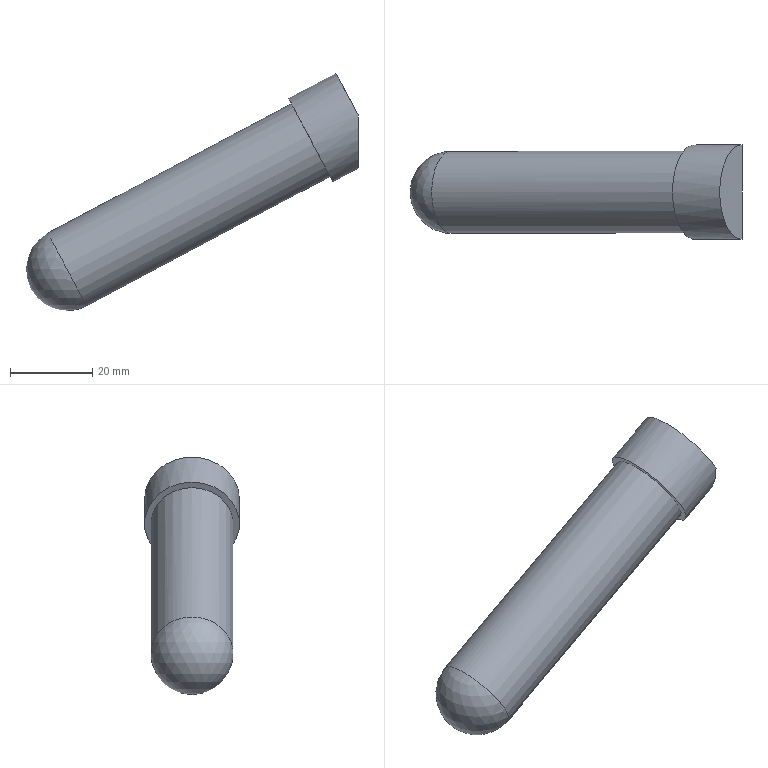Part | STEP file | solid 244 | 1 solid | 6 faces | box 80.636 x 23 x 57.712 mm | volume 28005 mm3 | plane 3 | cylinder 2 | sphere 1 | commonest cylinder face diameters 20 x1 23 x1